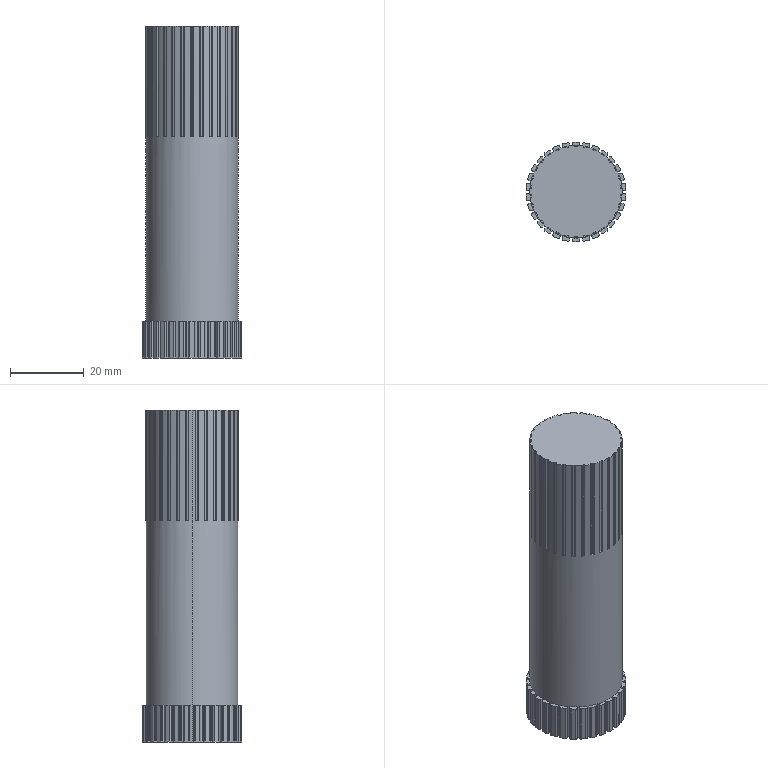Part | SolidWorks | features CirPattern 2, ICE 2, Extrusion 1 | 1 solid | 392 faces | box 26.982 x 27 x 90 mm | volume 44504 mm3 | plane 242 | cylinder 150 | commonest cylinder face diameters 0.4 x74 0.8 x74 25 x2